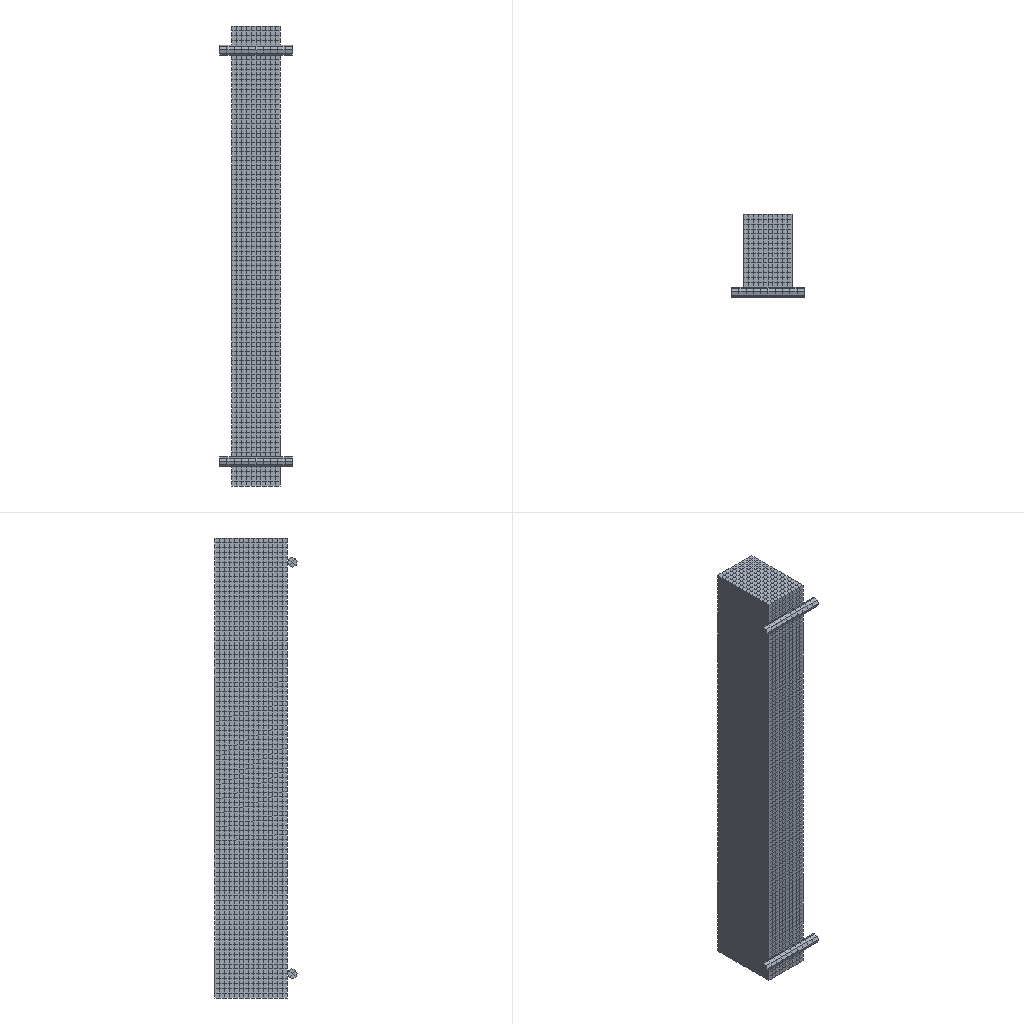Simulation study | abaqus
Set-up summary:
category,name,step,type,value,unit,region
solver,abaqus
solver,version,,,Abaqus/Standard 2020
units,not stated in the deck,,not stated
analysis,deck,,static,static
load_step,Step-1,Step-1,static
load_step,requested,,,1
mesh,nodes,,,17614
mesh,elements,,,14894
element_type,T3D2,,truss,414
element_type,C3D8R,,solid,14480
load,load commands in deck,,count,2
bc,support commands in deck,,count,1
material,CON,,in results
material,JIN,,in results
check,setup vs results,,match,"per instance, exact: element labels, types and connectivity; labels of the nodes the elements use; coordinates of those nodes at SINGLE_PRECISION in 3 of 4 instance(s)"
Abaqus input file, long lists of numbers shortened:
*Heading
** Job name: Job-1 Model name: Model-1
** Generated by: Abaqus/CAE 2020
*Preprint, echo=NO, model=NO, history=NO, contact=NO
**
** PARTS
**
*Part, name=Con
*Node
      1,         100.,         150.,         575.
      2,         100.,        -150.,         575.
** (17070 more lines like these left out)
*Element, type=C3D8R
   1,  136, 1079, 5859,  953,    1,   35,  757,   76
   2, 1079, 1080, 5860, 5859,   35,   36,  758,  757
** (14398 more lines like these left out)
*Nset, nset=Set-1, generate
     1,  17072,      1
*Elset, elset=Set-1, generate
     1,  14400,      1
** Section: con
*Solid Section, elset=Set-1, material=con
,
*End Part
**
*Part, name=jin
*Node
      1,    3814.1,        -200.,        -150.
      2,    3814.1,        -200.,        -100.
** (340 more lines like these left out)
*Element, type=T3D2
1, 1, 2
2, 2, 3
** (412 more lines like these left out)
*Nset, nset=Set-1, generate
   1,  342,    1
*Elset, elset=Set-1, generate
   1,  414,    1
** Section: jin
*Solid Section, elset=Set-1, material=jin
78.5,
*End Part
**
*Part, name=rigid
*Node
      1,  -2.209,  -19.878,         300.
      2,  -15.617,  -12.494,         300.
** (97 more lines like these left out)
*Element, type=C3D8R
 1, 10, 17, 18, 11,  1,  8,  9,  2
 2, 16, 15, 18, 17,  7,  6,  9,  8
** (38 more lines like these left out)
*Node
    100,           0., -1.2246468e-15,         300.
*Nset, nset=rigid-RefPt_, internal
100,
*Nset, nset=Set-1, generate
  1,  99,   1
*Elset, elset=Set-1, generate
  1,  40,   1
** Section: rig
*Solid Section, elset=Set-1, material=jin
,
*End Part
**
**
** ASSEMBLY
**
*Assembly, name=Assembly
**
*Instance, name=jin-1, part=jin
-50.,         100.,       -3450.
-50.,         100.,       -3450., -50., 99.,       -3450., 90.
*End Instance
**
*Instance, name=Con-1, part=Con
*End Instance
**
*Instance, name=rigid-1, part=rigid
       -150.,        -170.,         100.
       -150.,        -170.,         100.,        -150., -169.,         100., 90.
*End Instance
**
*Instance, name=rigid-2, part=rigid
       -150.,        -170.,        1800.
       -150.,        -170.,        1800.,        -150., -169.,        1800., 90.
*End Instance
**
*Node
      1,         150.,        -170.,         950.
*Node
      2,           0.,         150.,         950.
*Node
      3,           0.,         150.,        1400.
*Node
      4,           0.,         150.,         500.
*Nset, nset=Set-5
 1,
*Nset, nset=Set-7
 2,
*Nset, nset=Set-10
 3,
*Nset, nset=Set-11
 4,
*Nset, nset=b_Set-3, instance=rigid-1, generate
  1,  99,   1
*Nset, nset=b_Set-3, instance=rigid-2, generate
  1,  99,   1
*Elset, elset=b_Set-3, instance=rigid-1, generate
  1,  40,   1
*Elset, elset=b_Set-3, instance=rigid-2, generate
  1,  40,   1
*Nset, nset=m_Set-1, instance=jin-1, generate
   1,  342,    1
*Elset, elset=m_Set-1, instance=jin-1, generate
   1,  414,    1
*Nset, nset=m_Set-6
 2,
*Nset, nset=m_Set-8
 3,
*Nset, nset=m_Set-9
 4,
*Nset, nset=s_Set-1, instance=Con-1, generate
     1,  17072,      1
*Elset, elset=s_Set-1, instance=Con-1, generate
     1,  14400,      1
*Nset, nset=_PickedSet117, internal
 1,
*Elset, elset=_m_Surf-1_S3, internal, instance=rigid-1
  1,  2,  3,  5,  6,  7,  9, 10, 11, 13, 14, 15, 17, 18, 19, 21
 22, 23, 25, 26, 27, 29, 30, 31, 33, 34, 35, 37, 38, 39
*Elset, elset=_m_Surf-1_S3, internal, instance=rigid-2
  1,  2,  3,  5,  6,  7,  9, 10, 11, 13, 14, 15, 17, 18, 19, 21
 22, 23, 25, 26, 27, 29, 30, 31, 33, 34, 35, 37, 38, 39
*Elset, elset=_m_Surf-1_S6, internal, instance=rigid-1
  1,  2,  3,  5,  6,  7,  9, 10, 11, 13, 14, 15, 17, 18, 19, 21
 22, 23, 25, 26, 27, 29, 30, 31, 33, 34, 35, 37, 38, 39
*Elset, elset=_m_Surf-1_S6, internal, instance=rigid-2
  1,  2,  3,  5,  6,  7,  9, 10, 11, 13, 14, 15, 17, 18, 19, 21
 22, 23, 25, 26, 27, 29, 30, 31, 33, 34, 35, 37, 38, 39
*Elset, elset=_m_Surf-1_S4, internal, instance=rigid-1, generate
  4,  40,   4
*Elset, elset=_m_Surf-1_S4, internal, instance=rigid-2, generate
  4,  40,   4
*Elset, elset=_m_Surf-1_S5, internal, instance=rigid-1, generate
  4,  40,   4
*Elset, elset=_m_Surf-1_S5, internal, instance=rigid-2, generate
  4,  40,   4
*Surface, type=ELEMENT, name=m_Surf-1
_m_Surf-1_S3, S3
_m_Surf-1_S6, S6
_m_Surf-1_S4, S4
_m_Surf-1_S5, S5
*Elset, elset=_s_Surf-1_S4, internal, instance=Con-1
  2415,  2430,  2445,  2460,  2475,  2490,  2505,  2520,  2535,  2550,  2565,  2580,  2595,  2610,  2625,  2640
  2655,  2670,  2685,  2700,  2715,  2730,  2745,  2760,  2775,  2790,  2805,  2820,  2835,  2850,  2865,  2880
** (25 more lines like these left out)
*Surface, type=ELEMENT, name=s_Surf-1
_s_Surf-1_S4, S4
*Elset, elset=_s_Surf-3_S6, internal, instance=Con-1, generate
    1,  1186,    15
*Elset, elset=_s_Surf-3_S4, internal, instance=Con-1, generate
 1215,  2400,    15
*Surface, type=ELEMENT, name=s_Surf-3
_s_Surf-3_S6, S6
_s_Surf-3_S4, S4
*Elset, elset=_s_Surf-4_S4, internal, instance=Con-1, generate
 1215,  2400,    15
*Surface, type=ELEMENT, name=s_Surf-4
_s_Surf-4_S4, S4
*Elset, elset=_s_Surf-5_S6, internal, instance=Con-1, generate
    1,  1186,    15
*Surface, type=ELEMENT, name=s_Surf-5
_s_Surf-5_S6, S6
** Constraint: Constraint-1
*Embedded Element, host elset=s_Set-1
m_Set-1
** Constraint: Constraint-2
*Rigid Body, ref node=_PickedSet117, elset=b_Set-3, position=CENTER OF MASS
** Constraint: Constraint-3
*Coupling, constraint name=Constraint-3, ref node=m_Set-8, surface=s_Surf-4
*Kinematic
** Constraint: Constraint-4
*Coupling, constraint name=Constraint-4, ref node=m_Set-9, surface=s_Surf-5
*Kinematic
*End Assembly
*Amplitude, name=Amp-1
             0.,              0.,              1.,              1.
**
** MATERIALS
**
*Material, name=con
*Density
 2.2e-09,
*Elastic
29791., 0.2
*Concrete Damaged Plasticity
30.,    0.1,   1.16, 0.6667,   0.05
*Concrete Compression Hardening
 15.4,      0.
 16.9,  0.0002
 19.6, 0.00048
 20.1, 0.00079
  20., 0.00095
 19.6,  0.0011
 19.1, 0.00127
 18.6, 0.00143
 17.9,  0.0016
 17.2, 0.00177
 16.6, 0.00194
 15.9, 0.00211
 15.3, 0.00228
 14.7, 0.00245
 14.1, 0.00261
 13.5, 0.00278
  13., 0.00294
 12.5,  0.0031
  12., 0.00327
 11.6, 0.00343
 11.2, 0.00359
 10.8, 0.00375
 10.4, 0.00391
 10.1, 0.00406
*Concrete Tension Stiffening
 2.06,      0.
 1.92,   2e-05
 1.72,   4e-05
 1.53,   6e-05
 1.37,   8e-05
 1.24,  0.0001
 1.13, 0.00011
 1.04, 0.00013
 0.97, 0.00015
  0.9, 0.00016
 0.85, 0.00018
*Concrete Compression Damage
     0.,      0.
 0.0841,   9e-05
 0.0933,  0.0001
 0.1091, 0.00013
 0.1418,  0.0002
 0.2407, 0.00048
  0.322, 0.00079
 0.3557, 0.00095
 0.3886,  0.0011
 0.4201, 0.00127
 0.4499, 0.00143
 0.4778,  0.0016
 0.5039, 0.00177
 0.5282, 0.00194
 0.5506, 0.00211
 0.5715, 0.00228
 0.5908, 0.00245
 0.6086, 0.00261
 0.6252, 0.00278
 0.6406, 0.00294
 0.6549,  0.0031
 0.6682, 0.00327
 0.6806, 0.00343
 0.6922, 0.00359
  0.703, 0.00375
 0.7131, 0.00391
 0.7227, 0.00406
   0.74, 0.00438
 0.7554, 0.00469
 0.7691,   0.005
 0.7815, 0.00531
 0.7926, 0.00561
 0.8026, 0.00592
 0.8118, 0.00622
 0.8202, 0.00653
 0.8278, 0.00683
 0.8349, 0.00713
*Concrete Tension Damage
      0.,      0.
 0.1181,   2e-05
 0.2281,   4e-05
 0.3187,   6e-05
 0.3919,   8e-05
 0.4512,  0.0001
 0.5, 0.00011
  0.5407, 0.00013
 0.575, 0.00015
 0.6043, 0.00016
 0.6297, 0.00018
 0.7177, 0.00025
 0.7702, 0.00033
 0.8053,  0.0004
 0.8304, 0.00047
 0.8494, 0.00054
  0.8643, 0.00061
 0.8763, 0.00068
 0.8862, 0.00075
*Material, name=jin
*Density
 7.8e-09,
*Elastic
210000., 0.3
*Plastic
300.,0.
**
** INTERACTION PROPERTIES
**
*Surface Interaction, name=IntProp-1
1.,
*Friction, slip tolerance=0.005
 0.3,
*Surface Behavior, pressure-overclosure=HARD
**
** INTERACTIONS
**
** Interaction: Int-1
*Contact Pair, interaction=IntProp-1, type=SURFACE TO SURFACE
s_Surf-1, m_Surf-1
** ----------------------------------------------------------------
**
** STEP: Step-1
**
*Step, name=Step-1, nlgeom=YES, inc=1000
*Static, stabilize=0.0002, allsdtol=0.05, continue=NO
0.001, 1., 1e-06, 1.
**
** BOUNDARY CONDITIONS
**
** Name: BC-1 Type: 对称/反对称/完全固定
*Boundary
Set-5, ENCASTRE
**
** LOADS
**
** Name: Load-1   Type: Concentrated force
*Cload, amplitude=Amp-1
Set-10, 2, -80000.
** Name: Load-1-Copy   Type: Concentrated force
*Cload, amplitude=Amp-1
Set-11, 2, -80000.
**
** OUTPUT REQUESTS
**
*Restart, write, frequency=0
**
** FIELD OUTPUT: F-Output-1
**
*Output, field
*Node Output
CF, RF, U, V
*Element Output, directions=YES
DAMAGEC, DAMAGET, E, LE, MISES, MISESMAX, PE, PEEQ, PEMAG, S, SDEG, SSAVG
*Contact Output
CDISP, CSTRESS
**
** HISTORY OUTPUT: H-Output-2
**
*Output, history
*Node Output, nset=Set-10
U1, U2, U3
**
** HISTORY OUTPUT: H-Output-1
**
*Node Output, nset=Set-5
RF1, RF2, RF3
*End Step
Results summary:
result,step,,completed,increments=62 time=1.0/1.0
result,analysis,,,static
result,last_loadstep,,,1
result,primary field,,,U
result,reaction total,,FX,-0.000898,model units
result,reaction total,,FY,160000.0,model units
result,reaction total,,FZ,-0.0,model units